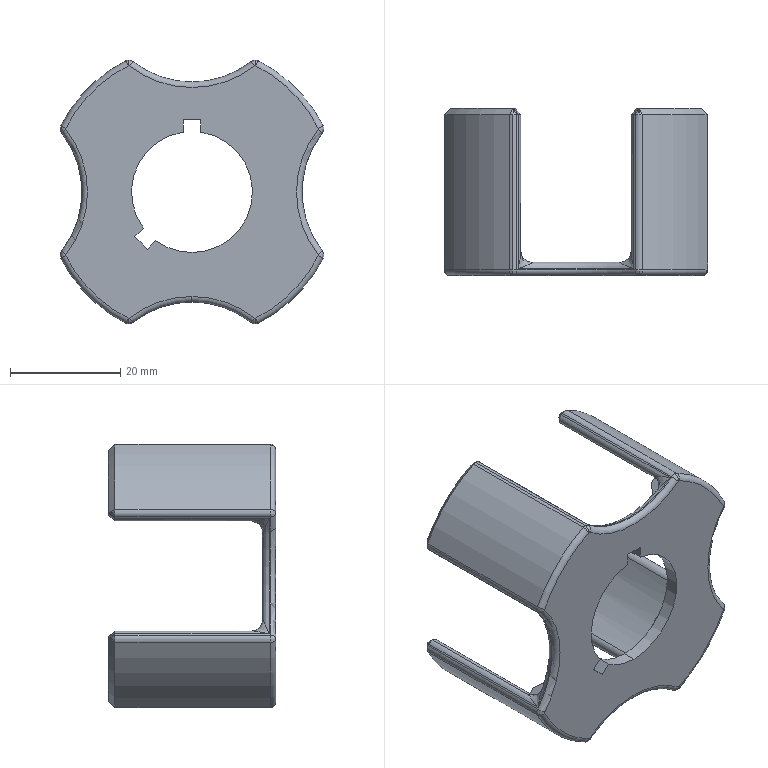Part | STEP file | Emergency stop protective ring J-V | 1 solid | 152 faces | box 47.915 x 30.4 x 47.915 mm | volume 9284 mm3 | cylinder 36 | torus 34 | plane 32 | cone 22 | spline 16 | other 12 | commonest cylinder face diameters 2.4 x20 35 x5 48 x4 53.4 x4 22 x3